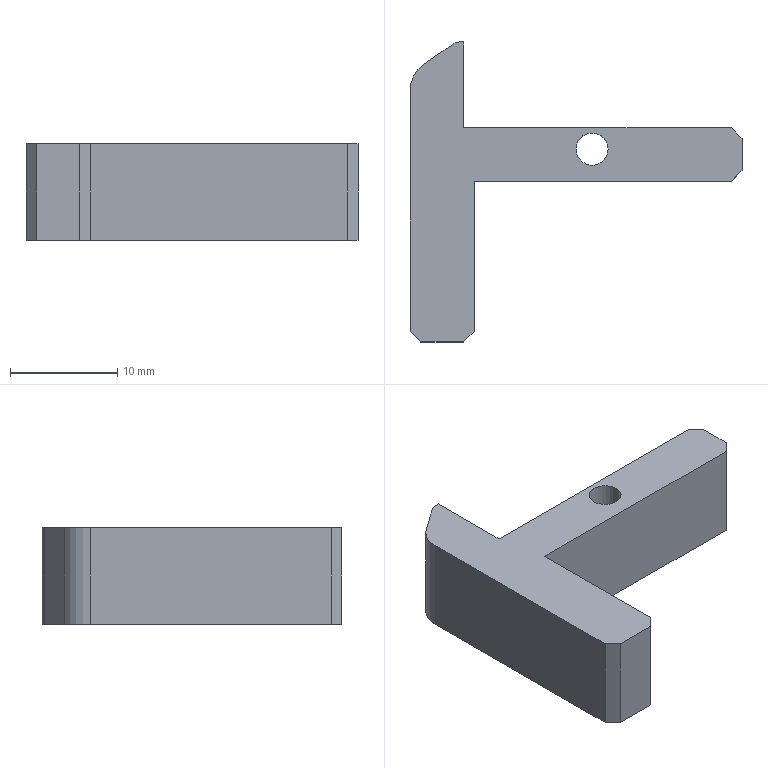Part | NX | features BREP 1 | 1 solid | 19 faces | box 31 x 28 x 9 mm | volume 2422 mm3 | plane 15 | cylinder 4 | commonest cylinder face diameters 3 x2 2 x1 6 x1
STEP:
#1=CARTESIAN_POINT('',(13.5,0.5,-4.5));
#2=VERTEX_POINT('',#1);
#3=CARTESIAN_POINT('',(10.5,0.5,-4.5));
#4=VERTEX_POINT('',#3);
#5=CARTESIAN_POINT('',(12.,0.5,-4.5));
#6=DIRECTION('',(0.,0.,-1.));
#7=DIRECTION('',(-1.,0.,0.));
#8=AXIS2_PLACEMENT_3D('',#5,#6,#7);
#9=CIRCLE('',#8,1.5);
#10=EDGE_CURVE('',#2,#4,#9,.T.);
#11=ORIENTED_EDGE('',*,*,#10,.T.);
#12=CARTESIAN_POINT('',(10.5,0.5,4.5));
#13=VERTEX_POINT('',#12);
#14=CARTESIAN_POINT('',(10.5,0.5,-5.5));
#15=DIRECTION('',(0.,0.,1.));
#16=VECTOR('',#15,1000.);
#17=LINE('',#14,#16);
#18=EDGE_CURVE('',#13,#4,#17,.F.);
#19=ORIENTED_EDGE('',*,*,#18,.F.);
#20=CARTESIAN_POINT('',(13.5,0.5,4.5));
#21=VERTEX_POINT('',#20);
#22=CARTESIAN_POINT('',(12.,0.5,4.5));
#23=DIRECTION('',(0.,0.,1.));
#24=DIRECTION('',(1.,0.,0.));
#25=AXIS2_PLACEMENT_3D('',#22,#23,#24);
#26=CIRCLE('',#25,1.5);
#27=EDGE_CURVE('',#13,#21,#26,.T.);
#28=ORIENTED_EDGE('',*,*,#27,.T.);
#29=CARTESIAN_POINT('',(13.5,0.5,-5.5));
#30=DIRECTION('',(0.,0.,1.));
#31=VECTOR('',#30,1000.);
#32=LINE('',#29,#31);
#33=EDGE_CURVE('',#21,#2,#32,.F.);
#34=ORIENTED_EDGE('',*,*,#33,.T.);
#35=EDGE_LOOP('',(#11,#19,#28,#34));
#36=FACE_BOUND('',#35,.T.);
#37=CARTESIAN_POINT('',(12.,0.5,-5.5));
#38=DIRECTION('',(0.,0.,1.));
#39=DIRECTION('',(1.,0.,0.));
#40=AXIS2_PLACEMENT_3D('',#37,#38,#39);
#41=CYLINDRICAL_SURFACE('',#40,1.5);
#42=ADVANCED_FACE('',(#36),#41,.F.);
#43=CARTESIAN_POINT('',(1.,-2.5,-4.5));
#44=VERTEX_POINT('',#43);
#45=CARTESIAN_POINT('',(25.,-2.5,-4.5));
#46=VERTEX_POINT('',#45);
#47=CARTESIAN_POINT('',(-5.,-2.5,-4.5));
#48=DIRECTION('',(1.,0.,0.));
#49=VECTOR('',#48,1000.);
#50=LINE('',#47,#49);
#51=EDGE_CURVE('',#44,#46,#50,.T.);
#52=ORIENTED_EDGE('',*,*,#51,.T.);
#53=CARTESIAN_POINT('',(25.,-2.5,4.5));
#54=VERTEX_POINT('',#53);
#55=CARTESIAN_POINT('',(25.,-2.5,4.5));
#56=DIRECTION('',(0.,0.,1.));
#57=VECTOR('',#56,1000.);
#58=LINE('',#55,#57);
#59=EDGE_CURVE('',#46,#54,#58,.T.);
#60=ORIENTED_EDGE('',*,*,#59,.T.);
#61=CARTESIAN_POINT('',(1.,-2.5,4.5));
#62=VERTEX_POINT('',#61);
#63=CARTESIAN_POINT('',(-5.,-2.5,4.5));
#64=DIRECTION('',(1.,0.,0.));
#65=VECTOR('',#64,1000.);
#66=LINE('',#63,#65);
#67=EDGE_CURVE('',#62,#54,#66,.T.);
#68=ORIENTED_EDGE('',*,*,#67,.F.);
#69=CARTESIAN_POINT('',(1.,-2.5,-4.5));
#70=DIRECTION('',(0.,0.,1.));
#71=VECTOR('',#70,1000.);
#72=LINE('',#69,#71);
#73=EDGE_CURVE('',#44,#62,#72,.T.);
#74=ORIENTED_EDGE('',*,*,#73,.F.);
#75=EDGE_LOOP('',(#52,#60,#68,#74));
#76=FACE_BOUND('',#75,.T.);
#77=CARTESIAN_POINT('',(-5.,-2.5,4.5));
#78=DIRECTION('',(0.,1.,0.));
#79=DIRECTION('',(1.,0.,0.));
#80=AXIS2_PLACEMENT_3D('',#77,#78,#79);
#81=PLANE('',#80);
#82=ADVANCED_FACE('',(#76),#81,.F.);
#83=CARTESIAN_POINT('',(25.,2.5,4.5));
#84=VERTEX_POINT('',#83);
#85=CARTESIAN_POINT('',(0.,2.5,4.5));
#86=VERTEX_POINT('',#85);
#87=CARTESIAN_POINT('',(0.,2.5,4.5));
#88=DIRECTION('',(-1.,0.,0.));
#89=VECTOR('',#88,1000.);
#90=LINE('',#87,#89);
#91=EDGE_CURVE('',#84,#86,#90,.T.);
#92=ORIENTED_EDGE('',*,*,#91,.F.);
#93=CARTESIAN_POINT('',(25.,2.5,-4.5));
#94=VERTEX_POINT('',#93);
#95=CARTESIAN_POINT('',(25.,2.5,4.5));
#96=DIRECTION('',(0.,0.,-1.));
#97=VECTOR('',#96,1000.);
#98=LINE('',#95,#97);
#99=EDGE_CURVE('',#84,#94,#98,.T.);
#100=ORIENTED_EDGE('',*,*,#99,.T.);
#101=CARTESIAN_POINT('',(0.,2.5,-4.5));
#102=VERTEX_POINT('',#101);
#103=CARTESIAN_POINT('',(0.,2.5,-4.5));
#104=DIRECTION('',(-1.,0.,0.));
#105=VECTOR('',#104,1000.);
#106=LINE('',#103,#105);
#107=EDGE_CURVE('',#94,#102,#106,.T.);
#108=ORIENTED_EDGE('',*,*,#107,.T.);
#109=CARTESIAN_POINT('',(0.,2.5,4.5));
#110=DIRECTION('',(0.,0.,-1.));
#111=VECTOR('',#110,1000.);
#112=LINE('',#109,#111);
#113=EDGE_CURVE('',#86,#102,#112,.T.);
#114=ORIENTED_EDGE('',*,*,#113,.F.);
#115=EDGE_LOOP('',(#92,#100,#108,#114));
#116=FACE_BOUND('',#115,.T.);
#117=CARTESIAN_POINT('',(0.,2.5,4.5));
#118=DIRECTION('',(0.,-1.,0.));
#119=DIRECTION('',(0.,0.,-1.));
#120=AXIS2_PLACEMENT_3D('',#117,#118,#119);
#121=PLANE('',#120);
#122=ADVANCED_FACE('',(#116),#121,.F.);
#123=CARTESIAN_POINT('',(0.,10.5,-4.5));
#124=VERTEX_POINT('',#123);
#125=CARTESIAN_POINT('',(0.,2.5,-4.5));
#126=DIRECTION('',(0.,1.,0.));
#127=VECTOR('',#126,1000.);
#128=LINE('',#125,#127);
#129=EDGE_CURVE('',#102,#124,#128,.T.);
#130=ORIENTED_EDGE('',*,*,#129,.T.);
#131=CARTESIAN_POINT('',(0.,10.5,4.5));
#132=VERTEX_POINT('',#131);
#133=CARTESIAN_POINT('',(0.,10.5,4.5));
#134=DIRECTION('',(0.,0.,-1.));
#135=VECTOR('',#134,1000.);
#136=LINE('',#133,#135);
#137=EDGE_CURVE('',#132,#124,#136,.T.);
#138=ORIENTED_EDGE('',*,*,#137,.F.);
#139=CARTESIAN_POINT('',(0.,2.5,4.5));
#140=DIRECTION('',(0.,1.,0.));
#141=VECTOR('',#140,1000.);
#142=LINE('',#139,#141);
#143=EDGE_CURVE('',#86,#132,#142,.T.);
#144=ORIENTED_EDGE('',*,*,#143,.F.);
#145=ORIENTED_EDGE('',*,*,#113,.T.);
#146=EDGE_LOOP('',(#130,#138,#144,#145));
#147=FACE_BOUND('',#146,.T.);
#148=CARTESIAN_POINT('',(0.,2.5,4.5));
#149=DIRECTION('',(-1.,0.,0.));
#150=DIRECTION('',(0.,0.,1.));
#151=AXIS2_PLACEMENT_3D('',#148,#149,#150);
#152=PLANE('',#151);
#153=ADVANCED_FACE('',(#147),#152,.F.);
#154=CARTESIAN_POINT('',(-0.4003,10.5,-4.5));
#155=VERTEX_POINT('',#154);
#156=CARTESIAN_POINT('',(0.,10.5,-4.5));
#157=DIRECTION('',(-1.,0.,0.));
#158=VECTOR('',#157,1000.);
#159=LINE('',#156,#158);
#160=EDGE_CURVE('',#124,#155,#159,.T.);
#161=ORIENTED_EDGE('',*,*,#160,.T.);
#162=CARTESIAN_POINT('',(-0.4003,10.5,4.5));
#163=VERTEX_POINT('',#162);
#164=CARTESIAN_POINT('',(-0.4003,10.5,4.5));
#165=DIRECTION('',(0.,0.,1.));
#166=VECTOR('',#165,1000.);
#167=LINE('',#164,#166);
#168=EDGE_CURVE('',#155,#163,#167,.T.);
#169=ORIENTED_EDGE('',*,*,#168,.T.);
#170=CARTESIAN_POINT('',(0.,10.5,4.5));
#171=DIRECTION('',(-1.,0.,0.));
#172=VECTOR('',#171,1000.);
#173=LINE('',#170,#172);
#174=EDGE_CURVE('',#132,#163,#173,.T.);
#175=ORIENTED_EDGE('',*,*,#174,.F.);
#176=ORIENTED_EDGE('',*,*,#137,.T.);
#177=EDGE_LOOP('',(#161,#169,#175,#176));
#178=FACE_BOUND('',#177,.T.);
#179=CARTESIAN_POINT('',(0.,10.5,4.5));
#180=DIRECTION('',(0.,-1.,0.));
#181=DIRECTION('',(0.,0.,-1.));
#182=AXIS2_PLACEMENT_3D('',#179,#180,#181);
#183=PLANE('',#182);
#184=ADVANCED_FACE('',(#178),#183,.F.);
#185=CARTESIAN_POINT('',(-5.,5.938,4.5));
#186=VERTEX_POINT('',#185);
#187=CARTESIAN_POINT('',(-5.,-16.5,4.5));
#188=VERTEX_POINT('',#187);
#189=CARTESIAN_POINT('',(-5.,10.5,4.5));
#190=DIRECTION('',(0.,-1.,0.));
#191=VECTOR('',#190,1000.);
#192=LINE('',#189,#191);
#193=EDGE_CURVE('',#186,#188,#192,.T.);
#194=ORIENTED_EDGE('',*,*,#193,.F.);
#195=CARTESIAN_POINT('',(-5.,5.938,-4.5));
#196=VERTEX_POINT('',#195);
#197=CARTESIAN_POINT('',(-5.,5.938,-4.5));
#198=DIRECTION('',(0.,0.,-1.));
#199=VECTOR('',#198,1000.);
#200=LINE('',#197,#199);
#201=EDGE_CURVE('',#186,#196,#200,.T.);
#202=ORIENTED_EDGE('',*,*,#201,.T.);
#203=CARTESIAN_POINT('',(-5.,-16.5,-4.5));
#204=VERTEX_POINT('',#203);
#205=CARTESIAN_POINT('',(-5.,10.5,-4.5));
#206=DIRECTION('',(0.,-1.,0.));
#207=VECTOR('',#206,1000.);
#208=LINE('',#205,#207);
#209=EDGE_CURVE('',#196,#204,#208,.T.);
#210=ORIENTED_EDGE('',*,*,#209,.T.);
#211=CARTESIAN_POINT('',(-5.,-16.5,4.5));
#212=DIRECTION('',(0.,0.,1.));
#213=VECTOR('',#212,1000.);
#214=LINE('',#211,#213);
#215=EDGE_CURVE('',#204,#188,#214,.T.);
#216=ORIENTED_EDGE('',*,*,#215,.T.);
#217=EDGE_LOOP('',(#194,#202,#210,#216));
#218=FACE_BOUND('',#217,.T.);
#219=CARTESIAN_POINT('',(-5.,10.5,4.5));
#220=DIRECTION('',(1.,0.,0.));
#221=DIRECTION('',(0.,1.,0.));
#222=AXIS2_PLACEMENT_3D('',#219,#220,#221);
#223=PLANE('',#222);
#224=ADVANCED_FACE('',(#218),#223,.F.);
#225=CARTESIAN_POINT('',(26.,-1.5,-4.5));
#226=VERTEX_POINT('',#225);
#227=CARTESIAN_POINT('',(26.,1.5,-4.5));
#228=VERTEX_POINT('',#227);
#229=CARTESIAN_POINT('',(26.,2.5,-4.5));
#230=DIRECTION('',(0.,1.,0.));
#231=VECTOR('',#230,1000.);
#232=LINE('',#229,#231);
#233=EDGE_CURVE('',#226,#228,#232,.T.);
#234=ORIENTED_EDGE('',*,*,#233,.T.);
#235=CARTESIAN_POINT('',(26.,1.5,4.5));
#236=VERTEX_POINT('',#235);
#237=CARTESIAN_POINT('',(26.,1.5,4.5));
#238=DIRECTION('',(0.,0.,1.));
#239=VECTOR('',#238,1000.);
#240=LINE('',#237,#239);
#241=EDGE_CURVE('',#228,#236,#240,.T.);
#242=ORIENTED_EDGE('',*,*,#241,.T.);
#243=CARTESIAN_POINT('',(26.,-1.5,4.5));
#244=VERTEX_POINT('',#243);
#245=CARTESIAN_POINT('',(26.,2.5,4.5));
#246=DIRECTION('',(0.,1.,0.));
#247=VECTOR('',#246,1000.);
#248=LINE('',#245,#247);
#249=EDGE_CURVE('',#244,#236,#248,.T.);
#250=ORIENTED_EDGE('',*,*,#249,.F.);
#251=CARTESIAN_POINT('',(26.,-1.5,4.5));
#252=DIRECTION('',(0.,0.,-1.));
#253=VECTOR('',#252,1000.);
#254=LINE('',#251,#253);
#255=EDGE_CURVE('',#244,#226,#254,.T.);
#256=ORIENTED_EDGE('',*,*,#255,.T.);
#257=EDGE_LOOP('',(#234,#242,#250,#256));
#258=FACE_BOUND('',#257,.T.);
#259=CARTESIAN_POINT('',(26.,2.5,4.5));
#260=DIRECTION('',(-1.,0.,0.));
#261=DIRECTION('',(0.,0.,1.));
#262=AXIS2_PLACEMENT_3D('',#259,#260,#261);
#263=PLANE('',#262);
#264=ADVANCED_FACE('',(#258),#263,.F.);
#265=CARTESIAN_POINT('',(-0.9738,10.319,4.5));
#266=VERTEX_POINT('',#265);
#267=CARTESIAN_POINT('',(-3.721,8.396,4.5));
#268=VERTEX_POINT('',#267);
#269=CARTESIAN_POINT('',(-5.,7.5,4.5));
#270=DIRECTION('',(-0.8192,-0.5736,0.));
#271=VECTOR('',#270,1000.);
#272=LINE('',#269,#271);
#273=EDGE_CURVE('',#266,#268,#272,.T.);
#274=ORIENTED_EDGE('',*,*,#273,.T.);
#275=CARTESIAN_POINT('',(-2.,5.938,4.5));
#276=DIRECTION('',(0.,0.,1.));
#277=DIRECTION('',(-1.,0.,0.));
#278=AXIS2_PLACEMENT_3D('',#275,#276,#277);
#279=CIRCLE('',#278,3.);
#280=EDGE_CURVE('',#268,#186,#279,.T.);
#281=ORIENTED_EDGE('',*,*,#280,.T.);
#282=ORIENTED_EDGE('',*,*,#193,.T.);
#283=CARTESIAN_POINT('',(-4.,-17.5,4.5));
#284=VERTEX_POINT('',#283);
#285=CARTESIAN_POINT('',(-5.,-16.5,4.5));
#286=DIRECTION('',(0.7071,-0.7071,0.));
#287=VECTOR('',#286,1000.);
#288=LINE('',#285,#287);
#289=EDGE_CURVE('',#188,#284,#288,.T.);
#290=ORIENTED_EDGE('',*,*,#289,.T.);
#291=CARTESIAN_POINT('',(0.,-17.5,4.5));
#292=VERTEX_POINT('',#291);
#293=CARTESIAN_POINT('',(-5.,-17.5,4.5));
#294=DIRECTION('',(1.,0.,0.));
#295=VECTOR('',#294,1000.);
#296=LINE('',#293,#295);
#297=EDGE_CURVE('',#284,#292,#296,.T.);
#298=ORIENTED_EDGE('',*,*,#297,.T.);
#299=CARTESIAN_POINT('',(1.,-16.5,4.5));
#300=VERTEX_POINT('',#299);
#301=CARTESIAN_POINT('',(0.,-17.5,4.5));
#302=DIRECTION('',(0.7071,0.7071,0.));
#303=VECTOR('',#302,1000.);
#304=LINE('',#301,#303);
#305=EDGE_CURVE('',#292,#300,#304,.T.);
#306=ORIENTED_EDGE('',*,*,#305,.T.);
#307=CARTESIAN_POINT('',(1.,-2.5,4.5));
#308=DIRECTION('',(0.,1.,0.));
#309=VECTOR('',#308,1000.);
#310=LINE('',#307,#309);
#311=EDGE_CURVE('',#300,#62,#310,.T.);
#312=ORIENTED_EDGE('',*,*,#311,.T.);
#313=ORIENTED_EDGE('',*,*,#67,.T.);
#314=CARTESIAN_POINT('',(26.,-1.5,4.5));
#315=DIRECTION('',(0.7071,0.7071,0.));
#316=VECTOR('',#315,1000.);
#317=LINE('',#314,#316);
#318=EDGE_CURVE('',#54,#244,#317,.T.);
#319=ORIENTED_EDGE('',*,*,#318,.T.);
#320=ORIENTED_EDGE('',*,*,#249,.T.);
#321=CARTESIAN_POINT('',(25.,2.5,4.5));
#322=DIRECTION('',(-0.7071,0.7071,0.));
#323=VECTOR('',#322,1000.);
#324=LINE('',#321,#323);
#325=EDGE_CURVE('',#236,#84,#324,.T.);
#326=ORIENTED_EDGE('',*,*,#325,.T.);
#327=ORIENTED_EDGE('',*,*,#91,.T.);
#328=ORIENTED_EDGE('',*,*,#143,.T.);
#329=ORIENTED_EDGE('',*,*,#174,.T.);
#330=CARTESIAN_POINT('',(-0.4003,9.5,4.5));
#331=DIRECTION('',(0.,0.,1.));
#332=DIRECTION('',(-1.,0.,0.));
#333=AXIS2_PLACEMENT_3D('',#330,#331,#332);
#334=CIRCLE('',#333,1.);
#335=EDGE_CURVE('',#163,#266,#334,.T.);
#336=ORIENTED_EDGE('',*,*,#335,.T.);
#337=EDGE_LOOP('',(#274,#281,#282,#290,#298,#306,#312,#313,#319,#320,#326,#327,#328,#329,#336));
#338=FACE_BOUND('',#337,.T.);
#339=CARTESIAN_POINT('',(12.,0.5,4.5));
#340=DIRECTION('',(0.,0.,1.));
#341=DIRECTION('',(1.,0.,0.));
#342=AXIS2_PLACEMENT_3D('',#339,#340,#341);
#343=CIRCLE('',#342,1.5);
#344=EDGE_CURVE('',#21,#13,#343,.T.);
#345=ORIENTED_EDGE('',*,*,#344,.F.);
#346=ORIENTED_EDGE('',*,*,#27,.F.);
#347=EDGE_LOOP('',(#345,#346));
#348=FACE_BOUND('',#347,.T.);
#349=CARTESIAN_POINT('',(26.,2.5,4.5));
#350=DIRECTION('',(0.,0.,-1.));
#351=DIRECTION('',(0.,-1.,0.));
#352=AXIS2_PLACEMENT_3D('',#349,#350,#351);
#353=PLANE('',#352);
#354=ADVANCED_FACE('',(#338,#348),#353,.F.);
#355=ORIENTED_EDGE('',*,*,#209,.F.);
#356=CARTESIAN_POINT('',(-3.721,8.396,-4.5));
#357=VERTEX_POINT('',#356);
#358=CARTESIAN_POINT('',(-2.,5.938,-4.5));
#359=DIRECTION('',(0.,0.,-1.));
#360=DIRECTION('',(-1.,0.,0.));
#361=AXIS2_PLACEMENT_3D('',#358,#359,#360);
#362=CIRCLE('',#361,3.);
#363=EDGE_CURVE('',#196,#357,#362,.T.);
#364=ORIENTED_EDGE('',*,*,#363,.T.);
#365=CARTESIAN_POINT('',(-0.9738,10.319,-4.5));
#366=VERTEX_POINT('',#365);
#367=CARTESIAN_POINT('',(13.452,20.42,-4.5));
#368=DIRECTION('',(0.8192,0.5736,0.));
#369=VECTOR('',#368,1000.);
#370=LINE('',#367,#369);
#371=EDGE_CURVE('',#357,#366,#370,.T.);
#372=ORIENTED_EDGE('',*,*,#371,.T.);
#373=CARTESIAN_POINT('',(-0.4003,9.5,-4.5));
#374=DIRECTION('',(0.,0.,-1.));
#375=DIRECTION('',(-1.,0.,0.));
#376=AXIS2_PLACEMENT_3D('',#373,#374,#375);
#377=CIRCLE('',#376,1.);
#378=EDGE_CURVE('',#366,#155,#377,.T.);
#379=ORIENTED_EDGE('',*,*,#378,.T.);
#380=ORIENTED_EDGE('',*,*,#160,.F.);
#381=ORIENTED_EDGE('',*,*,#129,.F.);
#382=ORIENTED_EDGE('',*,*,#107,.F.);
#383=CARTESIAN_POINT('',(25.5,2.,-4.5));
#384=DIRECTION('',(0.7071,-0.7071,0.));
#385=VECTOR('',#384,1000.);
#386=LINE('',#383,#385);
#387=EDGE_CURVE('',#94,#228,#386,.T.);
#388=ORIENTED_EDGE('',*,*,#387,.T.);
#389=ORIENTED_EDGE('',*,*,#233,.F.);
#390=CARTESIAN_POINT('',(28.,0.5,-4.5));
#391=DIRECTION('',(-0.7071,-0.7071,0.));
#392=VECTOR('',#391,1000.);
#393=LINE('',#390,#392);
#394=EDGE_CURVE('',#226,#46,#393,.T.);
#395=ORIENTED_EDGE('',*,*,#394,.T.);
#396=ORIENTED_EDGE('',*,*,#51,.F.);
#397=CARTESIAN_POINT('',(1.,-16.5,-4.5));
#398=VERTEX_POINT('',#397);
#399=CARTESIAN_POINT('',(1.,-2.5,-4.5));
#400=DIRECTION('',(0.,1.,0.));
#401=VECTOR('',#400,1000.);
#402=LINE('',#399,#401);
#403=EDGE_CURVE('',#398,#44,#402,.T.);
#404=ORIENTED_EDGE('',*,*,#403,.F.);
#405=CARTESIAN_POINT('',(0.,-17.5,-4.5));
#406=VERTEX_POINT('',#405);
#407=CARTESIAN_POINT('',(23.,5.5,-4.5));
#408=DIRECTION('',(-0.7071,-0.7071,0.));
#409=VECTOR('',#408,1000.);
#410=LINE('',#407,#409);
#411=EDGE_CURVE('',#398,#406,#410,.T.);
#412=ORIENTED_EDGE('',*,*,#411,.T.);
#413=CARTESIAN_POINT('',(-4.,-17.5,-4.5));
#414=VERTEX_POINT('',#413);
#415=CARTESIAN_POINT('',(-5.,-17.5,-4.5));
#416=DIRECTION('',(1.,0.,0.));
#417=VECTOR('',#416,1000.);
#418=LINE('',#415,#417);
#419=EDGE_CURVE('',#414,#406,#418,.T.);
#420=ORIENTED_EDGE('',*,*,#419,.F.);
#421=CARTESIAN_POINT('',(1.,-22.5,-4.5));
#422=DIRECTION('',(-0.7071,0.7071,0.));
#423=VECTOR('',#422,1000.);
#424=LINE('',#421,#423);
#425=EDGE_CURVE('',#414,#204,#424,.T.);
#426=ORIENTED_EDGE('',*,*,#425,.T.);
#427=EDGE_LOOP('',(#355,#364,#372,#379,#380,#381,#382,#388,#389,#395,#396,#404,#412,#420,#426));
#428=FACE_BOUND('',#427,.T.);
#429=ORIENTED_EDGE('',*,*,#10,.F.);
#430=CARTESIAN_POINT('',(12.,0.5,-4.5));
#431=DIRECTION('',(0.,0.,-1.));
#432=DIRECTION('',(-1.,0.,0.));
#433=AXIS2_PLACEMENT_3D('',#430,#431,#432);
#434=CIRCLE('',#433,1.5);
#435=EDGE_CURVE('',#4,#2,#434,.T.);
#436=ORIENTED_EDGE('',*,*,#435,.F.);
#437=EDGE_LOOP('',(#429,#436));
#438=FACE_BOUND('',#437,.T.);
#439=CARTESIAN_POINT('',(26.,2.5,-4.5));
#440=DIRECTION('',(0.,0.,-1.));
#441=DIRECTION('',(0.,-1.,0.));
#442=AXIS2_PLACEMENT_3D('',#439,#440,#441);
#443=PLANE('',#442);
#444=ADVANCED_FACE('',(#428,#438),#443,.T.);
#445=ORIENTED_EDGE('',*,*,#311,.F.);
#446=CARTESIAN_POINT('',(1.,-16.5,-4.5));
#447=DIRECTION('',(0.,0.,-1.));
#448=VECTOR('',#447,1000.);
#449=LINE('',#446,#448);
#450=EDGE_CURVE('',#300,#398,#449,.T.);
#451=ORIENTED_EDGE('',*,*,#450,.T.);
#452=ORIENTED_EDGE('',*,*,#403,.T.);
#453=ORIENTED_EDGE('',*,*,#73,.T.);
#454=EDGE_LOOP('',(#445,#451,#452,#453));
#455=FACE_BOUND('',#454,.T.);
#456=CARTESIAN_POINT('',(1.,-2.5,-4.5));
#457=DIRECTION('',(1.,0.,0.));
#458=DIRECTION('',(0.,1.,0.));
#459=AXIS2_PLACEMENT_3D('',#456,#457,#458);
#460=PLANE('',#459);
#461=ADVANCED_FACE('',(#455),#460,.T.);
#462=ORIENTED_EDGE('',*,*,#419,.T.);
#463=CARTESIAN_POINT('',(0.,-17.5,-4.5));
#464=DIRECTION('',(0.,0.,1.));
#465=VECTOR('',#464,1000.);
#466=LINE('',#463,#465);
#467=EDGE_CURVE('',#406,#292,#466,.T.);
#468=ORIENTED_EDGE('',*,*,#467,.T.);
#469=ORIENTED_EDGE('',*,*,#297,.F.);
#470=CARTESIAN_POINT('',(-4.,-17.5,-4.5));
#471=DIRECTION('',(0.,0.,-1.));
#472=VECTOR('',#471,1000.);
#473=LINE('',#470,#472);
#474=EDGE_CURVE('',#284,#414,#473,.T.);
#475=ORIENTED_EDGE('',*,*,#474,.T.);
#476=EDGE_LOOP('',(#462,#468,#469,#475));
#477=FACE_BOUND('',#476,.T.);
#478=CARTESIAN_POINT('',(-5.,-17.5,-4.5));
#479=DIRECTION('',(0.,-1.,0.));
#480=DIRECTION('',(0.,0.,-1.));
#481=AXIS2_PLACEMENT_3D('',#478,#479,#480);
#482=PLANE('',#481);
#483=ADVANCED_FACE('',(#477),#482,.T.);
#484=ORIENTED_EDGE('',*,*,#18,.T.);
#485=ORIENTED_EDGE('',*,*,#435,.T.);
#486=ORIENTED_EDGE('',*,*,#33,.F.);
#487=ORIENTED_EDGE('',*,*,#344,.T.);
#488=EDGE_LOOP('',(#484,#485,#486,#487));
#489=FACE_BOUND('',#488,.T.);
#490=CARTESIAN_POINT('',(12.,0.5,-5.5));
#491=DIRECTION('',(0.,0.,1.));
#492=DIRECTION('',(1.,0.,0.));
#493=AXIS2_PLACEMENT_3D('',#490,#491,#492);
#494=CYLINDRICAL_SURFACE('',#493,1.5);
#495=ADVANCED_FACE('',(#489),#494,.F.);
#496=ORIENTED_EDGE('',*,*,#325,.F.);
#497=ORIENTED_EDGE('',*,*,#241,.F.);
#498=ORIENTED_EDGE('',*,*,#387,.F.);
#499=ORIENTED_EDGE('',*,*,#99,.F.);
#500=EDGE_LOOP('',(#496,#497,#498,#499));
#501=FACE_BOUND('',#500,.T.);
#502=CARTESIAN_POINT('',(25.,2.5,4.5));
#503=DIRECTION('',(-0.7071,-0.7071,0.));
#504=DIRECTION('',(-0.7071,0.7071,0.));
#505=AXIS2_PLACEMENT_3D('',#502,#503,#504);
#506=PLANE('',#505);
#507=ADVANCED_FACE('',(#501),#506,.F.);
#508=ORIENTED_EDGE('',*,*,#318,.F.);
#509=ORIENTED_EDGE('',*,*,#59,.F.);
#510=ORIENTED_EDGE('',*,*,#394,.F.);
#511=ORIENTED_EDGE('',*,*,#255,.F.);
#512=EDGE_LOOP('',(#508,#509,#510,#511));
#513=FACE_BOUND('',#512,.T.);
#514=CARTESIAN_POINT('',(26.,-1.5,4.5));
#515=DIRECTION('',(-0.7071,0.7071,0.));
#516=DIRECTION('',(0.,0.,1.));
#517=AXIS2_PLACEMENT_3D('',#514,#515,#516);
#518=PLANE('',#517);
#519=ADVANCED_FACE('',(#513),#518,.F.);
#520=ORIENTED_EDGE('',*,*,#371,.F.);
#521=CARTESIAN_POINT('',(-3.721,8.396,4.5));
#522=DIRECTION('',(0.,0.,1.));
#523=VECTOR('',#522,1000.);
#524=LINE('',#521,#523);
#525=EDGE_CURVE('',#357,#268,#524,.T.);
#526=ORIENTED_EDGE('',*,*,#525,.T.);
#527=ORIENTED_EDGE('',*,*,#273,.F.);
#528=CARTESIAN_POINT('',(-0.9738,10.319,-4.5));
#529=DIRECTION('',(0.,0.,-1.));
#530=VECTOR('',#529,1000.);
#531=LINE('',#528,#530);
#532=EDGE_CURVE('',#266,#366,#531,.T.);
#533=ORIENTED_EDGE('',*,*,#532,.T.);
#534=EDGE_LOOP('',(#520,#526,#527,#533));
#535=FACE_BOUND('',#534,.T.);
#536=CARTESIAN_POINT('',(-5.,7.5,4.5));
#537=DIRECTION('',(0.5736,-0.8192,0.));
#538=DIRECTION('',(0.,0.,-1.));
#539=AXIS2_PLACEMENT_3D('',#536,#537,#538);
#540=PLANE('',#539);
#541=ADVANCED_FACE('',(#535),#540,.F.);
#542=ORIENTED_EDGE('',*,*,#378,.F.);
#543=ORIENTED_EDGE('',*,*,#532,.F.);
#544=ORIENTED_EDGE('',*,*,#335,.F.);
#545=ORIENTED_EDGE('',*,*,#168,.F.);
#546=EDGE_LOOP('',(#542,#543,#544,#545));
#547=FACE_BOUND('',#546,.T.);
#548=CARTESIAN_POINT('',(-0.4003,9.5,4.5));
#549=DIRECTION('',(0.,0.,1.));
#550=DIRECTION('',(1.,0.,0.));
#551=AXIS2_PLACEMENT_3D('',#548,#549,#550);
#552=CYLINDRICAL_SURFACE('',#551,1.);
#553=ADVANCED_FACE('',(#547),#552,.T.);
#554=ORIENTED_EDGE('',*,*,#411,.F.);
#555=ORIENTED_EDGE('',*,*,#450,.F.);
#556=ORIENTED_EDGE('',*,*,#305,.F.);
#557=ORIENTED_EDGE('',*,*,#467,.F.);
#558=EDGE_LOOP('',(#554,#555,#556,#557));
#559=FACE_BOUND('',#558,.T.);
#560=CARTESIAN_POINT('',(0.,-17.5,-4.5));
#561=DIRECTION('',(-0.7071,0.7071,0.));
#562=DIRECTION('',(0.,0.,1.));
#563=AXIS2_PLACEMENT_3D('',#560,#561,#562);
#564=PLANE('',#563);
#565=ADVANCED_FACE('',(#559),#564,.F.);
#566=ORIENTED_EDGE('',*,*,#425,.F.);
#567=ORIENTED_EDGE('',*,*,#474,.F.);
#568=ORIENTED_EDGE('',*,*,#289,.F.);
#569=ORIENTED_EDGE('',*,*,#215,.F.);
#570=EDGE_LOOP('',(#566,#567,#568,#569));
#571=FACE_BOUND('',#570,.T.);
#572=CARTESIAN_POINT('',(-5.,-16.5,4.5));
#573=DIRECTION('',(-0.7071,-0.7071,0.));
#574=DIRECTION('',(-0.7071,0.7071,0.));
#575=AXIS2_PLACEMENT_3D('',#572,#573,#574);
#576=PLANE('',#575);
#577=ADVANCED_FACE('',(#571),#576,.T.);
#578=ORIENTED_EDGE('',*,*,#280,.F.);
#579=ORIENTED_EDGE('',*,*,#525,.F.);
#580=ORIENTED_EDGE('',*,*,#363,.F.);
#581=ORIENTED_EDGE('',*,*,#201,.F.);
#582=EDGE_LOOP('',(#578,#579,#580,#581));
#583=FACE_BOUND('',#582,.T.);
#584=CARTESIAN_POINT('',(-2.,5.938,4.5));
#585=DIRECTION('',(0.,0.,-1.));
#586=DIRECTION('',(-1.,0.,0.));
#587=AXIS2_PLACEMENT_3D('',#584,#585,#586);
#588=CYLINDRICAL_SURFACE('',#587,3.);
#589=ADVANCED_FACE('',(#583),#588,.T.);
#590=CLOSED_SHELL('',(#42,#82,#122,#153,#184,#224,#264,#354,#444,#461,#483,#495,#507,#519,#541,#553,#565,#577,#589));
#591=MANIFOLD_SOLID_BREP('',#590);
#592=(LENGTH_UNIT()NAMED_UNIT(*)SI_UNIT(.MILLI.,.METRE.));
#593=UNCERTAINTY_MEASURE_WITH_UNIT(LENGTH_MEASURE(0.00001),#592,'','');
#594=(NAMED_UNIT(*)PLANE_ANGLE_UNIT()SI_UNIT($,.RADIAN.));
#595=(NAMED_UNIT(*)SI_UNIT($,.STERADIAN.)SOLID_ANGLE_UNIT());
#596=(GEOMETRIC_REPRESENTATION_CONTEXT(3)GLOBAL_UNCERTAINTY_ASSIGNED_CONTEXT((#593))GLOBAL_UNIT_ASSIGNED_CONTEXT((#592,#594,#595))REPRESENTATION_CONTEXT('',''));
#597=ADVANCED_BREP_SHAPE_REPRESENTATION('',(#591),#596);